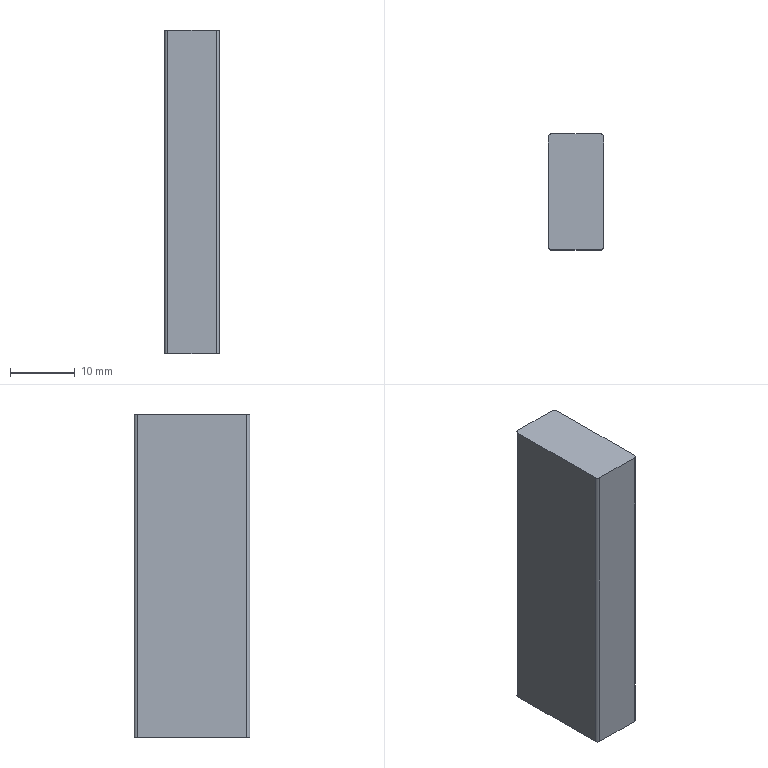Part | NX | features BREP 1 | 1 solid | 10 faces | box 8.52 x 17.946 x 50 mm | volume 7634 mm3 | plane 6 | cylinder 4 | commonest cylinder face diameters 1 x4
STEP:
#1=CARTESIAN_POINT('',(-3.76,8.973,-40.6));
#2=VERTEX_POINT('',#1);
#3=CARTESIAN_POINT('',(-4.26,8.473,-40.6));
#4=VERTEX_POINT('',#3);
#5=CARTESIAN_POINT('',(-3.76,8.473,-40.6));
#6=DIRECTION('',(0.,0.,1.));
#7=DIRECTION('',(1.,0.,0.));
#8=AXIS2_PLACEMENT_3D('',#5,#6,#7);
#9=CIRCLE('',#8,0.5);
#10=EDGE_CURVE('',#2,#4,#9,.T.);
#11=ORIENTED_EDGE('',*,*,#10,.F.);
#12=CARTESIAN_POINT('',(-3.76,8.973,-90.6));
#13=VERTEX_POINT('',#12);
#14=CARTESIAN_POINT('',(-3.76,8.973,-90.6));
#15=DIRECTION('',(0.,0.,1.));
#16=VECTOR('',#15,1000.);
#17=LINE('',#14,#16);
#18=EDGE_CURVE('',#13,#2,#17,.T.);
#19=ORIENTED_EDGE('',*,*,#18,.F.);
#20=CARTESIAN_POINT('',(-4.26,8.473,-90.6));
#21=VERTEX_POINT('',#20);
#22=CARTESIAN_POINT('',(-3.76,8.473,-90.6));
#23=DIRECTION('',(0.,0.,1.));
#24=DIRECTION('',(1.,0.,0.));
#25=AXIS2_PLACEMENT_3D('',#22,#23,#24);
#26=CIRCLE('',#25,0.5);
#27=EDGE_CURVE('',#13,#21,#26,.T.);
#28=ORIENTED_EDGE('',*,*,#27,.T.);
#29=CARTESIAN_POINT('',(-4.26,8.473,-90.6));
#30=DIRECTION('',(0.,0.,1.));
#31=VECTOR('',#30,1000.);
#32=LINE('',#29,#31);
#33=EDGE_CURVE('',#21,#4,#32,.T.);
#34=ORIENTED_EDGE('',*,*,#33,.T.);
#35=EDGE_LOOP('',(#11,#19,#28,#34));
#36=FACE_BOUND('',#35,.T.);
#37=CARTESIAN_POINT('',(-3.76,8.473,-90.6));
#38=DIRECTION('',(0.,0.,1.));
#39=DIRECTION('',(-1.,0.,0.));
#40=AXIS2_PLACEMENT_3D('',#37,#38,#39);
#41=CYLINDRICAL_SURFACE('',#40,0.5);
#42=ADVANCED_FACE('',(#36),#41,.T.);
#43=CARTESIAN_POINT('',(-4.26,-8.473,-40.6));
#44=VERTEX_POINT('',#43);
#45=CARTESIAN_POINT('',(-4.26,-8.473,-40.6));
#46=DIRECTION('',(0.,1.,0.));
#47=VECTOR('',#46,1000.);
#48=LINE('',#45,#47);
#49=EDGE_CURVE('',#44,#4,#48,.T.);
#50=ORIENTED_EDGE('',*,*,#49,.T.);
#51=ORIENTED_EDGE('',*,*,#33,.F.);
#52=CARTESIAN_POINT('',(-4.26,-8.473,-90.6));
#53=VERTEX_POINT('',#52);
#54=CARTESIAN_POINT('',(-4.26,-8.473,-90.6));
#55=DIRECTION('',(0.,1.,0.));
#56=VECTOR('',#55,1000.);
#57=LINE('',#54,#56);
#58=EDGE_CURVE('',#53,#21,#57,.T.);
#59=ORIENTED_EDGE('',*,*,#58,.F.);
#60=CARTESIAN_POINT('',(-4.26,-8.473,-90.6));
#61=DIRECTION('',(0.,0.,1.));
#62=VECTOR('',#61,1000.);
#63=LINE('',#60,#62);
#64=EDGE_CURVE('',#53,#44,#63,.T.);
#65=ORIENTED_EDGE('',*,*,#64,.T.);
#66=EDGE_LOOP('',(#50,#51,#59,#65));
#67=FACE_BOUND('',#66,.T.);
#68=CARTESIAN_POINT('',(-4.26,-8.473,-90.6));
#69=DIRECTION('',(1.,0.,0.));
#70=DIRECTION('',(0.,0.,1.));
#71=AXIS2_PLACEMENT_3D('',#68,#69,#70);
#72=PLANE('',#71);
#73=ADVANCED_FACE('',(#67),#72,.F.);
#74=CARTESIAN_POINT('',(-3.76,-8.973,-40.6));
#75=VERTEX_POINT('',#74);
#76=CARTESIAN_POINT('',(-3.76,-8.473,-40.6));
#77=DIRECTION('',(0.,0.,1.));
#78=DIRECTION('',(1.,0.,0.));
#79=AXIS2_PLACEMENT_3D('',#76,#77,#78);
#80=CIRCLE('',#79,0.5);
#81=EDGE_CURVE('',#44,#75,#80,.T.);
#82=ORIENTED_EDGE('',*,*,#81,.F.);
#83=ORIENTED_EDGE('',*,*,#64,.F.);
#84=CARTESIAN_POINT('',(-3.76,-8.973,-90.6));
#85=VERTEX_POINT('',#84);
#86=CARTESIAN_POINT('',(-3.76,-8.473,-90.6));
#87=DIRECTION('',(0.,0.,1.));
#88=DIRECTION('',(1.,0.,0.));
#89=AXIS2_PLACEMENT_3D('',#86,#87,#88);
#90=CIRCLE('',#89,0.5);
#91=EDGE_CURVE('',#53,#85,#90,.T.);
#92=ORIENTED_EDGE('',*,*,#91,.T.);
#93=CARTESIAN_POINT('',(-3.76,-8.973,-90.6));
#94=DIRECTION('',(0.,0.,1.));
#95=VECTOR('',#94,1000.);
#96=LINE('',#93,#95);
#97=EDGE_CURVE('',#85,#75,#96,.T.);
#98=ORIENTED_EDGE('',*,*,#97,.T.);
#99=EDGE_LOOP('',(#82,#83,#92,#98));
#100=FACE_BOUND('',#99,.T.);
#101=CARTESIAN_POINT('',(-3.76,-8.473,-90.6));
#102=DIRECTION('',(0.,0.,1.));
#103=DIRECTION('',(-1.,0.,0.));
#104=AXIS2_PLACEMENT_3D('',#101,#102,#103);
#105=CYLINDRICAL_SURFACE('',#104,0.5);
#106=ADVANCED_FACE('',(#100),#105,.T.);
#107=CARTESIAN_POINT('',(3.76,-8.973,-40.6));
#108=VERTEX_POINT('',#107);
#109=CARTESIAN_POINT('',(3.76,-8.973,-40.6));
#110=DIRECTION('',(-1.,0.,0.));
#111=VECTOR('',#110,1000.);
#112=LINE('',#109,#111);
#113=EDGE_CURVE('',#108,#75,#112,.T.);
#114=ORIENTED_EDGE('',*,*,#113,.T.);
#115=ORIENTED_EDGE('',*,*,#97,.F.);
#116=CARTESIAN_POINT('',(3.76,-8.973,-90.6));
#117=VERTEX_POINT('',#116);
#118=CARTESIAN_POINT('',(3.76,-8.973,-90.6));
#119=DIRECTION('',(-1.,0.,0.));
#120=VECTOR('',#119,1000.);
#121=LINE('',#118,#120);
#122=EDGE_CURVE('',#117,#85,#121,.T.);
#123=ORIENTED_EDGE('',*,*,#122,.F.);
#124=CARTESIAN_POINT('',(3.76,-8.973,-90.6));
#125=DIRECTION('',(0.,0.,1.));
#126=VECTOR('',#125,1000.);
#127=LINE('',#124,#126);
#128=EDGE_CURVE('',#117,#108,#127,.T.);
#129=ORIENTED_EDGE('',*,*,#128,.T.);
#130=EDGE_LOOP('',(#114,#115,#123,#129));
#131=FACE_BOUND('',#130,.T.);
#132=CARTESIAN_POINT('',(3.76,-8.973,-90.6));
#133=DIRECTION('',(0.,1.,0.));
#134=DIRECTION('',(0.,0.,-1.));
#135=AXIS2_PLACEMENT_3D('',#132,#133,#134);
#136=PLANE('',#135);
#137=ADVANCED_FACE('',(#131),#136,.F.);
#138=CARTESIAN_POINT('',(4.26,-8.473,-40.6));
#139=VERTEX_POINT('',#138);
#140=CARTESIAN_POINT('',(3.76,-8.473,-40.6));
#141=DIRECTION('',(0.,0.,1.));
#142=DIRECTION('',(1.,0.,0.));
#143=AXIS2_PLACEMENT_3D('',#140,#141,#142);
#144=CIRCLE('',#143,0.5);
#145=EDGE_CURVE('',#108,#139,#144,.T.);
#146=ORIENTED_EDGE('',*,*,#145,.F.);
#147=ORIENTED_EDGE('',*,*,#128,.F.);
#148=CARTESIAN_POINT('',(4.26,-8.473,-90.6));
#149=VERTEX_POINT('',#148);
#150=CARTESIAN_POINT('',(3.76,-8.473,-90.6));
#151=DIRECTION('',(0.,0.,1.));
#152=DIRECTION('',(1.,0.,0.));
#153=AXIS2_PLACEMENT_3D('',#150,#151,#152);
#154=CIRCLE('',#153,0.5);
#155=EDGE_CURVE('',#117,#149,#154,.T.);
#156=ORIENTED_EDGE('',*,*,#155,.T.);
#157=CARTESIAN_POINT('',(4.26,-8.473,-90.6));
#158=DIRECTION('',(0.,0.,1.));
#159=VECTOR('',#158,1000.);
#160=LINE('',#157,#159);
#161=EDGE_CURVE('',#149,#139,#160,.T.);
#162=ORIENTED_EDGE('',*,*,#161,.T.);
#163=EDGE_LOOP('',(#146,#147,#156,#162));
#164=FACE_BOUND('',#163,.T.);
#165=CARTESIAN_POINT('',(3.76,-8.473,-90.6));
#166=DIRECTION('',(0.,0.,1.));
#167=DIRECTION('',(-1.,0.,0.));
#168=AXIS2_PLACEMENT_3D('',#165,#166,#167);
#169=CYLINDRICAL_SURFACE('',#168,0.5);
#170=ADVANCED_FACE('',(#164),#169,.T.);
#171=CARTESIAN_POINT('',(4.26,8.473,-40.6));
#172=VERTEX_POINT('',#171);
#173=CARTESIAN_POINT('',(4.26,8.473,-40.6));
#174=DIRECTION('',(0.,-1.,0.));
#175=VECTOR('',#174,1000.);
#176=LINE('',#173,#175);
#177=EDGE_CURVE('',#172,#139,#176,.T.);
#178=ORIENTED_EDGE('',*,*,#177,.T.);
#179=ORIENTED_EDGE('',*,*,#161,.F.);
#180=CARTESIAN_POINT('',(4.26,8.473,-90.6));
#181=VERTEX_POINT('',#180);
#182=CARTESIAN_POINT('',(4.26,8.473,-90.6));
#183=DIRECTION('',(0.,-1.,0.));
#184=VECTOR('',#183,1000.);
#185=LINE('',#182,#184);
#186=EDGE_CURVE('',#181,#149,#185,.T.);
#187=ORIENTED_EDGE('',*,*,#186,.F.);
#188=CARTESIAN_POINT('',(4.26,8.473,-90.6));
#189=DIRECTION('',(0.,0.,1.));
#190=VECTOR('',#189,1000.);
#191=LINE('',#188,#190);
#192=EDGE_CURVE('',#181,#172,#191,.T.);
#193=ORIENTED_EDGE('',*,*,#192,.T.);
#194=EDGE_LOOP('',(#178,#179,#187,#193));
#195=FACE_BOUND('',#194,.T.);
#196=CARTESIAN_POINT('',(4.26,8.473,-90.6));
#197=DIRECTION('',(-1.,0.,0.));
#198=DIRECTION('',(0.,1.,0.));
#199=AXIS2_PLACEMENT_3D('',#196,#197,#198);
#200=PLANE('',#199);
#201=ADVANCED_FACE('',(#195),#200,.F.);
#202=CARTESIAN_POINT('',(3.76,8.973,-40.6));
#203=VERTEX_POINT('',#202);
#204=CARTESIAN_POINT('',(3.76,8.473,-40.6));
#205=DIRECTION('',(0.,0.,1.));
#206=DIRECTION('',(1.,0.,0.));
#207=AXIS2_PLACEMENT_3D('',#204,#205,#206);
#208=CIRCLE('',#207,0.5);
#209=EDGE_CURVE('',#172,#203,#208,.T.);
#210=ORIENTED_EDGE('',*,*,#209,.F.);
#211=ORIENTED_EDGE('',*,*,#192,.F.);
#212=CARTESIAN_POINT('',(3.76,8.973,-90.6));
#213=VERTEX_POINT('',#212);
#214=CARTESIAN_POINT('',(3.76,8.473,-90.6));
#215=DIRECTION('',(0.,0.,1.));
#216=DIRECTION('',(1.,0.,0.));
#217=AXIS2_PLACEMENT_3D('',#214,#215,#216);
#218=CIRCLE('',#217,0.5);
#219=EDGE_CURVE('',#181,#213,#218,.T.);
#220=ORIENTED_EDGE('',*,*,#219,.T.);
#221=CARTESIAN_POINT('',(3.76,8.973,-90.6));
#222=DIRECTION('',(0.,0.,1.));
#223=VECTOR('',#222,1000.);
#224=LINE('',#221,#223);
#225=EDGE_CURVE('',#213,#203,#224,.T.);
#226=ORIENTED_EDGE('',*,*,#225,.T.);
#227=EDGE_LOOP('',(#210,#211,#220,#226));
#228=FACE_BOUND('',#227,.T.);
#229=CARTESIAN_POINT('',(3.76,8.473,-90.6));
#230=DIRECTION('',(0.,0.,1.));
#231=DIRECTION('',(-1.,0.,0.));
#232=AXIS2_PLACEMENT_3D('',#229,#230,#231);
#233=CYLINDRICAL_SURFACE('',#232,0.5);
#234=ADVANCED_FACE('',(#228),#233,.T.);
#235=CARTESIAN_POINT('',(-3.76,8.973,-40.6));
#236=DIRECTION('',(1.,0.,0.));
#237=VECTOR('',#236,1000.);
#238=LINE('',#235,#237);
#239=EDGE_CURVE('',#2,#203,#238,.T.);
#240=ORIENTED_EDGE('',*,*,#239,.T.);
#241=ORIENTED_EDGE('',*,*,#225,.F.);
#242=CARTESIAN_POINT('',(-3.76,8.973,-90.6));
#243=DIRECTION('',(1.,0.,0.));
#244=VECTOR('',#243,1000.);
#245=LINE('',#242,#244);
#246=EDGE_CURVE('',#13,#213,#245,.T.);
#247=ORIENTED_EDGE('',*,*,#246,.F.);
#248=ORIENTED_EDGE('',*,*,#18,.T.);
#249=EDGE_LOOP('',(#240,#241,#247,#248));
#250=FACE_BOUND('',#249,.T.);
#251=CARTESIAN_POINT('',(-3.76,8.973,-90.6));
#252=DIRECTION('',(0.,-1.,0.));
#253=DIRECTION('',(-1.,0.,0.));
#254=AXIS2_PLACEMENT_3D('',#251,#252,#253);
#255=PLANE('',#254);
#256=ADVANCED_FACE('',(#250),#255,.F.);
#257=ORIENTED_EDGE('',*,*,#27,.F.);
#258=ORIENTED_EDGE('',*,*,#246,.T.);
#259=ORIENTED_EDGE('',*,*,#219,.F.);
#260=ORIENTED_EDGE('',*,*,#186,.T.);
#261=ORIENTED_EDGE('',*,*,#155,.F.);
#262=ORIENTED_EDGE('',*,*,#122,.T.);
#263=ORIENTED_EDGE('',*,*,#91,.F.);
#264=ORIENTED_EDGE('',*,*,#58,.T.);
#265=EDGE_LOOP('',(#257,#258,#259,#260,#261,#262,#263,#264));
#266=FACE_BOUND('',#265,.T.);
#267=CARTESIAN_POINT('',(-3.76,8.473,-90.6));
#268=DIRECTION('',(0.,0.,1.));
#269=DIRECTION('',(-1.,0.,0.));
#270=AXIS2_PLACEMENT_3D('',#267,#268,#269);
#271=PLANE('',#270);
#272=ADVANCED_FACE('',(#266),#271,.F.);
#273=ORIENTED_EDGE('',*,*,#10,.T.);
#274=ORIENTED_EDGE('',*,*,#49,.F.);
#275=ORIENTED_EDGE('',*,*,#81,.T.);
#276=ORIENTED_EDGE('',*,*,#113,.F.);
#277=ORIENTED_EDGE('',*,*,#145,.T.);
#278=ORIENTED_EDGE('',*,*,#177,.F.);
#279=ORIENTED_EDGE('',*,*,#209,.T.);
#280=ORIENTED_EDGE('',*,*,#239,.F.);
#281=EDGE_LOOP('',(#273,#274,#275,#276,#277,#278,#279,#280));
#282=FACE_BOUND('',#281,.T.);
#283=CARTESIAN_POINT('',(-3.76,8.473,-40.6));
#284=DIRECTION('',(0.,0.,1.));
#285=DIRECTION('',(-1.,0.,0.));
#286=AXIS2_PLACEMENT_3D('',#283,#284,#285);
#287=PLANE('',#286);
#288=ADVANCED_FACE('',(#282),#287,.T.);
#289=CLOSED_SHELL('',(#42,#73,#106,#137,#170,#201,#234,#256,#272,#288));
#290=MANIFOLD_SOLID_BREP('',#289);
#291=(LENGTH_UNIT()NAMED_UNIT(*)SI_UNIT(.MILLI.,.METRE.));
#292=UNCERTAINTY_MEASURE_WITH_UNIT(LENGTH_MEASURE(0.00001),#291,'','');
#293=(NAMED_UNIT(*)PLANE_ANGLE_UNIT()SI_UNIT($,.RADIAN.));
#294=(NAMED_UNIT(*)SI_UNIT($,.STERADIAN.)SOLID_ANGLE_UNIT());
#295=(GEOMETRIC_REPRESENTATION_CONTEXT(3)GLOBAL_UNCERTAINTY_ASSIGNED_CONTEXT((#292))GLOBAL_UNIT_ASSIGNED_CONTEXT((#291,#293,#294))REPRESENTATION_CONTEXT('',''));
#296=ADVANCED_BREP_SHAPE_REPRESENTATION('',(#290),#295);